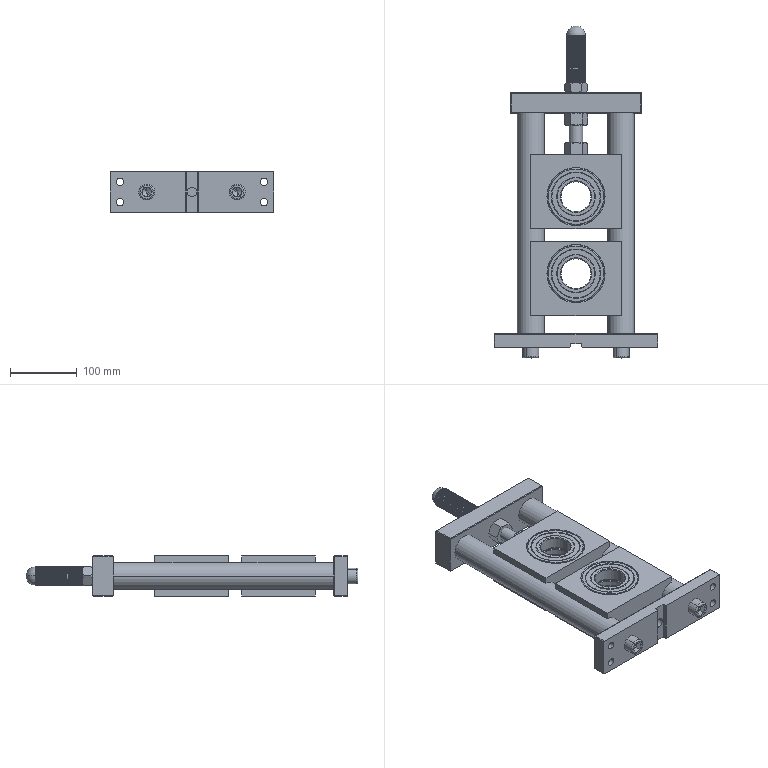Part | SolidWorks | 93 solids | 1849 faces | box 245 x 496 x 60 mm | volume 2710635 mm3 | cylinder 810 | plane 359 | torus 306 | sphere 274 | cone 100 | commonest cylinder face diameters 0.5 x360 63 x124 67 x124 28 x60 40 x18 58.333 x16